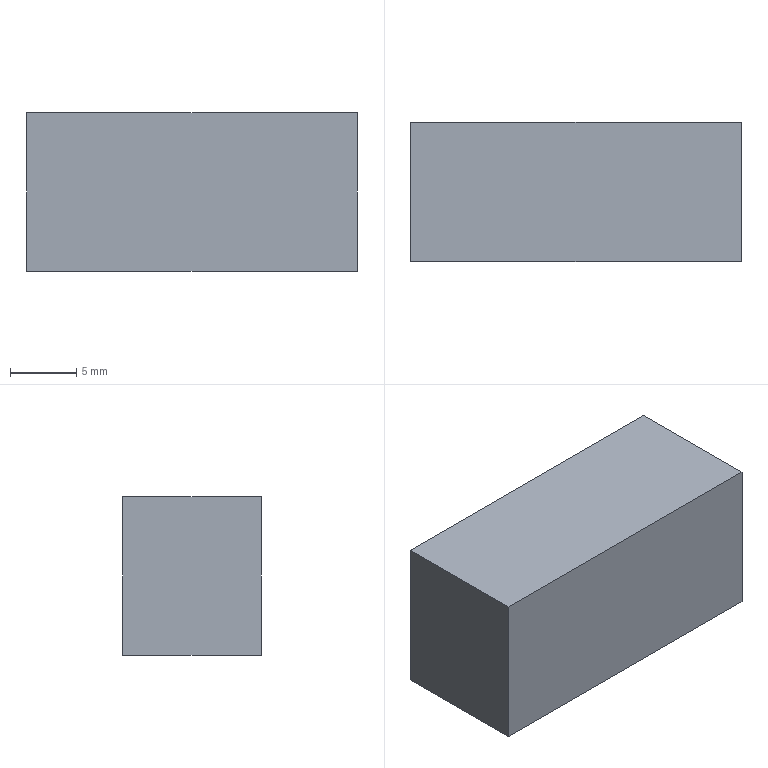Part | SolidWorks | features Extrusion 1 | 1 solid | 6 faces | box 25 x 10.5 x 12 mm | volume 3150 mm3 | plane 6
STEP:
#1=CARTESIAN_POINT('',(-12.5,5.25,6.));
#2=VERTEX_POINT('',#1);
#3=CARTESIAN_POINT('',(-12.5,-5.25,6.));
#4=VERTEX_POINT('',#3);
#5=CARTESIAN_POINT('',(-12.5,5.25,6.));
#6=DIRECTION('',(0.,-1.,0.));
#7=VECTOR('',#6,1000.);
#8=LINE('',#5,#7);
#9=EDGE_CURVE('',#2,#4,#8,.T.);
#10=ORIENTED_EDGE('',*,*,#9,.F.);
#11=CARTESIAN_POINT('',(-12.5,5.25,-6.));
#12=VERTEX_POINT('',#11);
#13=CARTESIAN_POINT('',(-12.5,5.25,-6.));
#14=DIRECTION('',(0.,0.,1.));
#15=VECTOR('',#14,1000.);
#16=LINE('',#13,#15);
#17=EDGE_CURVE('',#12,#2,#16,.T.);
#18=ORIENTED_EDGE('',*,*,#17,.F.);
#19=CARTESIAN_POINT('',(-12.5,-5.25,-6.));
#20=VERTEX_POINT('',#19);
#21=CARTESIAN_POINT('',(-12.5,5.25,-6.));
#22=DIRECTION('',(0.,-1.,0.));
#23=VECTOR('',#22,1000.);
#24=LINE('',#21,#23);
#25=EDGE_CURVE('',#12,#20,#24,.T.);
#26=ORIENTED_EDGE('',*,*,#25,.T.);
#27=CARTESIAN_POINT('',(-12.5,-5.25,-6.));
#28=DIRECTION('',(0.,0.,1.));
#29=VECTOR('',#28,1000.);
#30=LINE('',#27,#29);
#31=EDGE_CURVE('',#20,#4,#30,.T.);
#32=ORIENTED_EDGE('',*,*,#31,.T.);
#33=EDGE_LOOP('',(#10,#18,#26,#32));
#34=FACE_OUTER_BOUND('',#33,.T.);
#35=CARTESIAN_POINT('',(-12.5,5.25,-6.));
#36=DIRECTION('',(-1.,0.,0.));
#37=DIRECTION('',(0.,0.,1.));
#38=AXIS2_PLACEMENT_3D('',#35,#36,#37);
#39=PLANE('',#38);
#40=ADVANCED_FACE('',(#34),#39,.T.);
#41=CARTESIAN_POINT('',(12.5,5.25,6.));
#42=VERTEX_POINT('',#41);
#43=CARTESIAN_POINT('',(12.5,5.25,6.));
#44=DIRECTION('',(-1.,0.,0.));
#45=VECTOR('',#44,1000.);
#46=LINE('',#43,#45);
#47=EDGE_CURVE('',#42,#2,#46,.T.);
#48=ORIENTED_EDGE('',*,*,#47,.F.);
#49=CARTESIAN_POINT('',(12.5,5.25,-6.));
#50=VERTEX_POINT('',#49);
#51=CARTESIAN_POINT('',(12.5,5.25,-6.));
#52=DIRECTION('',(0.,0.,1.));
#53=VECTOR('',#52,1000.);
#54=LINE('',#51,#53);
#55=EDGE_CURVE('',#50,#42,#54,.T.);
#56=ORIENTED_EDGE('',*,*,#55,.F.);
#57=CARTESIAN_POINT('',(12.5,5.25,-6.));
#58=DIRECTION('',(-1.,0.,0.));
#59=VECTOR('',#58,1000.);
#60=LINE('',#57,#59);
#61=EDGE_CURVE('',#50,#12,#60,.T.);
#62=ORIENTED_EDGE('',*,*,#61,.T.);
#63=ORIENTED_EDGE('',*,*,#17,.T.);
#64=EDGE_LOOP('',(#48,#56,#62,#63));
#65=FACE_OUTER_BOUND('',#64,.T.);
#66=CARTESIAN_POINT('',(12.5,5.25,-6.));
#67=DIRECTION('',(0.,1.,0.));
#68=DIRECTION('',(0.,0.,1.));
#69=AXIS2_PLACEMENT_3D('',#66,#67,#68);
#70=PLANE('',#69);
#71=ADVANCED_FACE('',(#65),#70,.T.);
#72=CARTESIAN_POINT('',(12.5,-5.25,6.));
#73=VERTEX_POINT('',#72);
#74=CARTESIAN_POINT('',(12.5,-5.25,6.));
#75=DIRECTION('',(0.,1.,0.));
#76=VECTOR('',#75,1000.);
#77=LINE('',#74,#76);
#78=EDGE_CURVE('',#73,#42,#77,.T.);
#79=ORIENTED_EDGE('',*,*,#78,.F.);
#80=CARTESIAN_POINT('',(12.5,-5.25,-6.));
#81=VERTEX_POINT('',#80);
#82=CARTESIAN_POINT('',(12.5,-5.25,-6.));
#83=DIRECTION('',(0.,0.,1.));
#84=VECTOR('',#83,1000.);
#85=LINE('',#82,#84);
#86=EDGE_CURVE('',#81,#73,#85,.T.);
#87=ORIENTED_EDGE('',*,*,#86,.F.);
#88=CARTESIAN_POINT('',(12.5,-5.25,-6.));
#89=DIRECTION('',(0.,1.,0.));
#90=VECTOR('',#89,1000.);
#91=LINE('',#88,#90);
#92=EDGE_CURVE('',#81,#50,#91,.T.);
#93=ORIENTED_EDGE('',*,*,#92,.T.);
#94=ORIENTED_EDGE('',*,*,#55,.T.);
#95=EDGE_LOOP('',(#79,#87,#93,#94));
#96=FACE_OUTER_BOUND('',#95,.T.);
#97=CARTESIAN_POINT('',(12.5,-5.25,-6.));
#98=DIRECTION('',(1.,0.,0.));
#99=DIRECTION('',(0.,0.,-1.));
#100=AXIS2_PLACEMENT_3D('',#97,#98,#99);
#101=PLANE('',#100);
#102=ADVANCED_FACE('',(#96),#101,.T.);
#103=CARTESIAN_POINT('',(-12.5,-5.25,6.));
#104=DIRECTION('',(1.,0.,0.));
#105=VECTOR('',#104,1000.);
#106=LINE('',#103,#105);
#107=EDGE_CURVE('',#4,#73,#106,.T.);
#108=ORIENTED_EDGE('',*,*,#107,.F.);
#109=ORIENTED_EDGE('',*,*,#31,.F.);
#110=CARTESIAN_POINT('',(-12.5,-5.25,-6.));
#111=DIRECTION('',(1.,0.,0.));
#112=VECTOR('',#111,1000.);
#113=LINE('',#110,#112);
#114=EDGE_CURVE('',#20,#81,#113,.T.);
#115=ORIENTED_EDGE('',*,*,#114,.T.);
#116=ORIENTED_EDGE('',*,*,#86,.T.);
#117=EDGE_LOOP('',(#108,#109,#115,#116));
#118=FACE_OUTER_BOUND('',#117,.T.);
#119=CARTESIAN_POINT('',(-12.5,-5.25,-6.));
#120=DIRECTION('',(0.,-1.,0.));
#121=DIRECTION('',(0.,0.,-1.));
#122=AXIS2_PLACEMENT_3D('',#119,#120,#121);
#123=PLANE('',#122);
#124=ADVANCED_FACE('',(#118),#123,.T.);
#125=ORIENTED_EDGE('',*,*,#25,.F.);
#126=ORIENTED_EDGE('',*,*,#61,.F.);
#127=ORIENTED_EDGE('',*,*,#92,.F.);
#128=ORIENTED_EDGE('',*,*,#114,.F.);
#129=EDGE_LOOP('',(#125,#126,#127,#128));
#130=FACE_OUTER_BOUND('',#129,.T.);
#131=CARTESIAN_POINT('',(0.,0.,-6.));
#132=DIRECTION('',(0.,0.,1.));
#133=DIRECTION('',(1.,0.,0.));
#134=AXIS2_PLACEMENT_3D('',#131,#132,#133);
#135=PLANE('',#134);
#136=ADVANCED_FACE('',(#130),#135,.F.);
#137=ORIENTED_EDGE('',*,*,#9,.T.);
#138=ORIENTED_EDGE('',*,*,#107,.T.);
#139=ORIENTED_EDGE('',*,*,#78,.T.);
#140=ORIENTED_EDGE('',*,*,#47,.T.);
#141=EDGE_LOOP('',(#137,#138,#139,#140));
#142=FACE_OUTER_BOUND('',#141,.T.);
#143=CARTESIAN_POINT('',(0.,0.,6.));
#144=DIRECTION('',(0.,0.,1.));
#145=DIRECTION('',(1.,0.,0.));
#146=AXIS2_PLACEMENT_3D('',#143,#144,#145);
#147=PLANE('',#146);
#148=ADVANCED_FACE('',(#142),#147,.T.);
#149=CLOSED_SHELL('',(#40,#71,#102,#124,#136,#148));
#150=MANIFOLD_SOLID_BREP('',#149);
#151=CARTESIAN_POINT('',(0.,0.,0.));
#152=DIRECTION('',(0.,0.,1.));
#153=DIRECTION('',(1.,0.,0.));
#154=AXIS2_PLACEMENT_3D('',#151,#152,#153);
#155=(LENGTH_UNIT()NAMED_UNIT(*)SI_UNIT(.MILLI.,.METRE.));
#156=UNCERTAINTY_MEASURE_WITH_UNIT(LENGTH_MEASURE(0.00001),#155,'','');
#157=(NAMED_UNIT(*)PLANE_ANGLE_UNIT()SI_UNIT($,.RADIAN.));
#158=(NAMED_UNIT(*)SI_UNIT($,.STERADIAN.)SOLID_ANGLE_UNIT());
#159=(GEOMETRIC_REPRESENTATION_CONTEXT(3)GLOBAL_UNCERTAINTY_ASSIGNED_CONTEXT((#156))GLOBAL_UNIT_ASSIGNED_CONTEXT((#155,#157,#158))REPRESENTATION_CONTEXT('',''));
#160=ADVANCED_BREP_SHAPE_REPRESENTATION('',(#150,#154),#159);